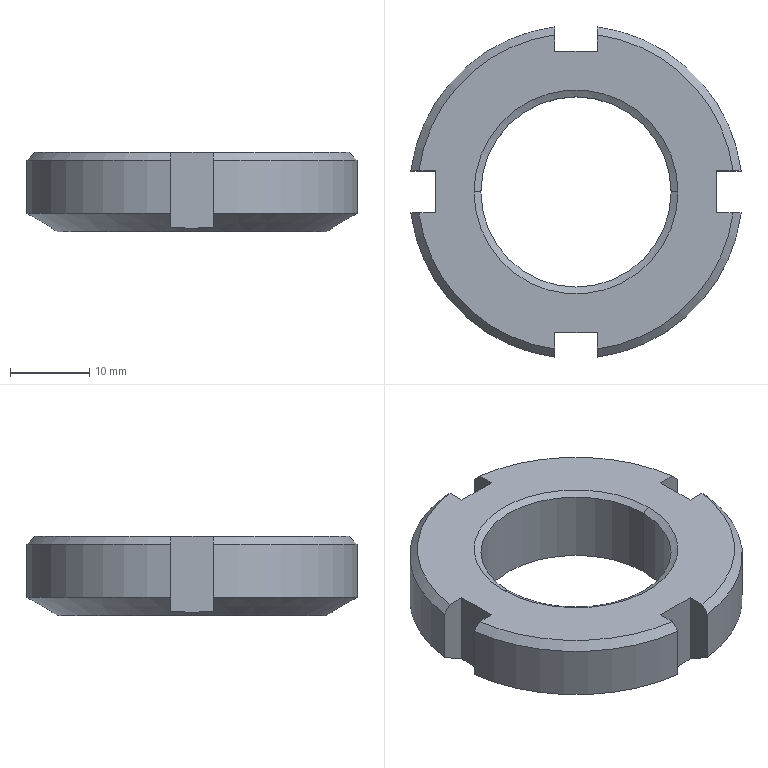Part | SolidWorks | features Chamfer 3, CirPattern 1, Cut 1, Extrusion 1 | 1 solid | 30 faces | box 41.664 x 41.664 x 10 mm | volume 8085 mm3 | plane 14 | cone 10 | cylinder 6 | commonest cylinder face diameters 42 x4 24 x2
STEP:
#1=CARTESIAN_POINT('',(-12.,0.,9.5));
#2=VERTEX_POINT('',#1);
#3=CARTESIAN_POINT('',(12.,0.,9.5));
#4=VERTEX_POINT('',#3);
#5=CARTESIAN_POINT('',(0.,0.,9.5));
#6=DIRECTION('',(0.,0.,1.));
#7=DIRECTION('',(1.,0.,0.));
#8=AXIS2_PLACEMENT_3D('',#5,#6,#7);
#9=CIRCLE('',#8,12.);
#10=EDGE_CURVE('',#2,#4,#9,.T.);
#11=ORIENTED_EDGE('',*,*,#10,.F.);
#12=CARTESIAN_POINT('',(-12.866,0.,10.));
#13=VERTEX_POINT('',#12);
#14=CARTESIAN_POINT('',(-12.,0.,9.5));
#15=DIRECTION('',(-0.866,0.,0.5));
#16=VECTOR('',#15,1000.);
#17=LINE('',#14,#16);
#18=EDGE_CURVE('',#2,#13,#17,.T.);
#19=ORIENTED_EDGE('',*,*,#18,.T.);
#20=CARTESIAN_POINT('',(12.866,0.,10.));
#21=VERTEX_POINT('',#20);
#22=CARTESIAN_POINT('',(0.,0.,10.));
#23=DIRECTION('',(0.,0.,-1.));
#24=DIRECTION('',(1.,0.,0.));
#25=AXIS2_PLACEMENT_3D('',#22,#23,#24);
#26=CIRCLE('',#25,12.866);
#27=EDGE_CURVE('',#21,#13,#26,.T.);
#28=ORIENTED_EDGE('',*,*,#27,.F.);
#29=CARTESIAN_POINT('',(12.,0.,9.5));
#30=DIRECTION('',(0.866,0.,0.5));
#31=VECTOR('',#30,1000.);
#32=LINE('',#29,#31);
#33=EDGE_CURVE('',#4,#21,#32,.T.);
#34=ORIENTED_EDGE('',*,*,#33,.F.);
#35=EDGE_LOOP('',(#11,#19,#28,#34));
#36=FACE_OUTER_BOUND('',#35,.T.);
#37=CARTESIAN_POINT('',(0.,0.,9.5));
#38=DIRECTION('',(0.,0.,1.));
#39=DIRECTION('',(1.,0.,0.));
#40=AXIS2_PLACEMENT_3D('',#37,#38,#39);
#41=CONICAL_SURFACE('',#40,12.,1.047);
#42=ADVANCED_FACE('',(#36),#41,.F.);
#43=CARTESIAN_POINT('',(12.,0.,0.5));
#44=VERTEX_POINT('',#43);
#45=CARTESIAN_POINT('',(-12.,0.,0.5));
#46=VERTEX_POINT('',#45);
#47=CARTESIAN_POINT('',(0.,0.,0.5));
#48=DIRECTION('',(0.,0.,-1.));
#49=DIRECTION('',(1.,0.,0.));
#50=AXIS2_PLACEMENT_3D('',#47,#48,#49);
#51=CIRCLE('',#50,12.);
#52=EDGE_CURVE('',#44,#46,#51,.T.);
#53=ORIENTED_EDGE('',*,*,#52,.F.);
#54=CARTESIAN_POINT('',(12.866,0.,0.));
#55=VERTEX_POINT('',#54);
#56=CARTESIAN_POINT('',(12.866,0.,0.));
#57=DIRECTION('',(0.866,0.,-0.5));
#58=VECTOR('',#57,1000.);
#59=LINE('',#56,#58);
#60=EDGE_CURVE('',#44,#55,#59,.T.);
#61=ORIENTED_EDGE('',*,*,#60,.T.);
#62=CARTESIAN_POINT('',(-12.866,0.,0.));
#63=VERTEX_POINT('',#62);
#64=CARTESIAN_POINT('',(0.,0.,0.));
#65=DIRECTION('',(0.,0.,1.));
#66=DIRECTION('',(1.,0.,0.));
#67=AXIS2_PLACEMENT_3D('',#64,#65,#66);
#68=CIRCLE('',#67,12.866);
#69=EDGE_CURVE('',#63,#55,#68,.T.);
#70=ORIENTED_EDGE('',*,*,#69,.F.);
#71=CARTESIAN_POINT('',(-12.866,0.,0.));
#72=DIRECTION('',(-0.866,0.,-0.5));
#73=VECTOR('',#72,1000.);
#74=LINE('',#71,#73);
#75=EDGE_CURVE('',#46,#63,#74,.T.);
#76=ORIENTED_EDGE('',*,*,#75,.F.);
#77=EDGE_LOOP('',(#53,#61,#70,#76));
#78=FACE_OUTER_BOUND('',#77,.T.);
#79=CARTESIAN_POINT('',(0.,0.,0.));
#80=DIRECTION('',(0.,0.,-1.));
#81=DIRECTION('',(-1.,0.,0.));
#82=AXIS2_PLACEMENT_3D('',#79,#80,#81);
#83=CONICAL_SURFACE('',#82,12.866,1.047);
#84=ADVANCED_FACE('',(#78),#83,.F.);
#85=CARTESIAN_POINT('',(-17.,0.,0.));
#86=VERTEX_POINT('',#85);
#87=CARTESIAN_POINT('',(17.,0.,0.));
#88=VERTEX_POINT('',#87);
#89=CARTESIAN_POINT('',(0.,0.,0.));
#90=DIRECTION('',(0.,0.,-1.));
#91=DIRECTION('',(1.,0.,0.));
#92=AXIS2_PLACEMENT_3D('',#89,#90,#91);
#93=CIRCLE('',#92,17.);
#94=EDGE_CURVE('',#86,#88,#93,.T.);
#95=ORIENTED_EDGE('',*,*,#94,.F.);
#96=CARTESIAN_POINT('',(-17.732,0.,0.4227));
#97=VERTEX_POINT('',#96);
#98=CARTESIAN_POINT('',(-21.,0.,2.309));
#99=DIRECTION('',(-0.866,0.,0.5));
#100=VECTOR('',#99,1000.);
#101=LINE('',#98,#100);
#102=EDGE_CURVE('',#86,#97,#101,.T.);
#103=ORIENTED_EDGE('',*,*,#102,.T.);
#104=CARTESIAN_POINT('',(-17.732,2.65,0.5364));
#105=VERTEX_POINT('',#104);
#106=CARTESIAN_POINT('',(-17.732,2.65,0.5364));
#107=CARTESIAN_POINT('',(-17.732,1.77,0.4613));
#108=CARTESIAN_POINT('',(-17.732,0.8867,0.4227));
#109=CARTESIAN_POINT('',(-17.732,0.,0.4227));
#110=B_SPLINE_CURVE_WITH_KNOTS('',3,(#106,#107,#108,#109),.UNSPECIFIED.,.F.,.F.,(4,4),(0.005044,0.007694),.UNSPECIFIED.);
#111=EDGE_CURVE('',#105,#97,#110,.T.);
#112=ORIENTED_EDGE('',*,*,#111,.F.);
#113=CARTESIAN_POINT('',(-20.832,2.65,2.309));
#114=VERTEX_POINT('',#113);
#115=CARTESIAN_POINT('',(-20.832,2.65,2.309));
#116=CARTESIAN_POINT('',(-19.799,2.65,1.718));
#117=CARTESIAN_POINT('',(-18.766,2.65,1.127));
#118=CARTESIAN_POINT('',(-17.732,2.65,0.5364));
#119=B_SPLINE_CURVE_WITH_KNOTS('',3,(#115,#116,#117,#118),.UNSPECIFIED.,.F.,.F.,(4,4),(0.00673,0.0103),.UNSPECIFIED.);
#120=EDGE_CURVE('',#114,#105,#119,.T.);
#121=ORIENTED_EDGE('',*,*,#120,.F.);
#122=CARTESIAN_POINT('',(-2.65,20.832,2.309));
#123=VERTEX_POINT('',#122);
#124=CARTESIAN_POINT('',(0.,0.,2.309));
#125=DIRECTION('',(0.,0.,1.));
#126=DIRECTION('',(1.,0.,0.));
#127=AXIS2_PLACEMENT_3D('',#124,#125,#126);
#128=CIRCLE('',#127,21.);
#129=EDGE_CURVE('',#123,#114,#128,.T.);
#130=ORIENTED_EDGE('',*,*,#129,.F.);
#131=CARTESIAN_POINT('',(-2.65,17.732,0.5364));
#132=VERTEX_POINT('',#131);
#133=CARTESIAN_POINT('',(-2.65,17.732,0.5364));
#134=CARTESIAN_POINT('',(-2.65,18.766,1.127));
#135=CARTESIAN_POINT('',(-2.65,19.799,1.718));
#136=CARTESIAN_POINT('',(-2.65,20.832,2.309));
#137=B_SPLINE_CURVE_WITH_KNOTS('',3,(#133,#134,#135,#136),.UNSPECIFIED.,.F.,.F.,(4,4),(0.006997,0.01057),.UNSPECIFIED.);
#138=EDGE_CURVE('',#132,#123,#137,.T.);
#139=ORIENTED_EDGE('',*,*,#138,.F.);
#140=CARTESIAN_POINT('',(2.65,17.732,0.5364));
#141=VERTEX_POINT('',#140);
#142=CARTESIAN_POINT('',(2.65,17.732,0.5364));
#143=CARTESIAN_POINT('',(1.773,17.732,0.4615));
#144=CARTESIAN_POINT('',(0.8926,17.732,0.423));
#145=CARTESIAN_POINT('',(-0.4329,17.732,0.4226));
#146=CARTESIAN_POINT('',(-0.8756,17.732,0.432));
#147=CARTESIAN_POINT('',(-1.763,17.732,0.47));
#148=CARTESIAN_POINT('',(-2.208,17.732,0.4986));
#149=CARTESIAN_POINT('',(-2.65,17.732,0.5364));
#150=B_SPLINE_CURVE_WITH_KNOTS('',3,(#142,#143,#144,#145,#146,#147,#148,#149),.UNSPECIFIED.,.F.,.F.,(4,2,2,4),(0.005044,0.007685,0.009006,0.01033),.UNSPECIFIED.);
#151=EDGE_CURVE('',#141,#132,#150,.T.);
#152=ORIENTED_EDGE('',*,*,#151,.F.);
#153=CARTESIAN_POINT('',(2.65,20.832,2.309));
#154=VERTEX_POINT('',#153);
#155=CARTESIAN_POINT('',(2.65,20.832,2.309));
#156=CARTESIAN_POINT('',(2.65,19.799,1.718));
#157=CARTESIAN_POINT('',(2.65,18.766,1.127));
#158=CARTESIAN_POINT('',(2.65,17.732,0.5364));
#159=B_SPLINE_CURVE_WITH_KNOTS('',3,(#155,#156,#157,#158),.UNSPECIFIED.,.F.,.F.,(4,4),(0.004139,0.00771),.UNSPECIFIED.);
#160=EDGE_CURVE('',#154,#141,#159,.T.);
#161=ORIENTED_EDGE('',*,*,#160,.F.);
#162=CARTESIAN_POINT('',(20.832,2.65,2.309));
#163=VERTEX_POINT('',#162);
#164=CARTESIAN_POINT('',(0.,0.,2.309));
#165=DIRECTION('',(0.,0.,1.));
#166=DIRECTION('',(1.,0.,0.));
#167=AXIS2_PLACEMENT_3D('',#164,#165,#166);
#168=CIRCLE('',#167,21.);
#169=EDGE_CURVE('',#163,#154,#168,.T.);
#170=ORIENTED_EDGE('',*,*,#169,.F.);
#171=CARTESIAN_POINT('',(17.732,2.65,0.5364));
#172=VERTEX_POINT('',#171);
#173=CARTESIAN_POINT('',(17.732,2.65,0.5364));
#174=CARTESIAN_POINT('',(18.766,2.65,1.127));
#175=CARTESIAN_POINT('',(19.799,2.65,1.718));
#176=CARTESIAN_POINT('',(20.832,2.65,2.309));
#177=B_SPLINE_CURVE_WITH_KNOTS('',3,(#173,#174,#175,#176),.UNSPECIFIED.,.F.,.F.,(4,4),(0.006997,0.01057),.UNSPECIFIED.);
#178=EDGE_CURVE('',#172,#163,#177,.T.);
#179=ORIENTED_EDGE('',*,*,#178,.F.);
#180=CARTESIAN_POINT('',(17.732,0.,0.4227));
#181=VERTEX_POINT('',#180);
#182=CARTESIAN_POINT('',(17.732,0.,0.4227));
#183=CARTESIAN_POINT('',(17.732,0.8867,0.4227));
#184=CARTESIAN_POINT('',(17.732,1.77,0.4613));
#185=CARTESIAN_POINT('',(17.732,2.65,0.5364));
#186=B_SPLINE_CURVE_WITH_KNOTS('',3,(#182,#183,#184,#185),.UNSPECIFIED.,.F.,.F.,(4,4),(0.01369,0.01634),.UNSPECIFIED.);
#187=EDGE_CURVE('',#181,#172,#186,.T.);
#188=ORIENTED_EDGE('',*,*,#187,.F.);
#189=CARTESIAN_POINT('',(21.,0.,2.309));
#190=DIRECTION('',(0.866,0.,0.5));
#191=VECTOR('',#190,1000.);
#192=LINE('',#189,#191);
#193=EDGE_CURVE('',#88,#181,#192,.T.);
#194=ORIENTED_EDGE('',*,*,#193,.F.);
#195=EDGE_LOOP('',(#95,#103,#112,#121,#130,#139,#152,#161,#170,#179,#188,#194));
#196=FACE_OUTER_BOUND('',#195,.T.);
#197=CARTESIAN_POINT('',(0.,0.,2.309));
#198=DIRECTION('',(0.,0.,1.));
#199=DIRECTION('',(1.,0.,0.));
#200=AXIS2_PLACEMENT_3D('',#197,#198,#199);
#201=CONICAL_SURFACE('',#200,21.,1.047);
#202=ADVANCED_FACE('',(#196),#201,.T.);
#203=ORIENTED_EDGE('',*,*,#10,.T.);
#204=CARTESIAN_POINT('',(12.,0.,10.));
#205=DIRECTION('',(0.,0.,-1.));
#206=VECTOR('',#205,1000.);
#207=LINE('',#204,#206);
#208=EDGE_CURVE('',#4,#44,#207,.T.);
#209=ORIENTED_EDGE('',*,*,#208,.T.);
#210=ORIENTED_EDGE('',*,*,#52,.T.);
#211=CARTESIAN_POINT('',(-12.,0.,10.));
#212=DIRECTION('',(0.,0.,-1.));
#213=VECTOR('',#212,1000.);
#214=LINE('',#211,#213);
#215=EDGE_CURVE('',#2,#46,#214,.T.);
#216=ORIENTED_EDGE('',*,*,#215,.F.);
#217=EDGE_LOOP('',(#203,#209,#210,#216));
#218=FACE_OUTER_BOUND('',#217,.T.);
#219=CARTESIAN_POINT('',(0.,0.,10.));
#220=DIRECTION('',(0.,0.,-1.));
#221=DIRECTION('',(-1.,0.,0.));
#222=AXIS2_PLACEMENT_3D('',#219,#220,#221);
#223=CYLINDRICAL_SURFACE('',#222,12.);
#224=ADVANCED_FACE('',(#218),#223,.F.);
#225=CARTESIAN_POINT('',(2.65,20.832,9.));
#226=VERTEX_POINT('',#225);
#227=CARTESIAN_POINT('',(20.832,2.65,9.));
#228=VERTEX_POINT('',#227);
#229=CARTESIAN_POINT('',(0.,0.,9.));
#230=DIRECTION('',(0.,0.,-1.));
#231=DIRECTION('',(1.,0.,0.));
#232=AXIS2_PLACEMENT_3D('',#229,#230,#231);
#233=CIRCLE('',#232,21.);
#234=EDGE_CURVE('',#226,#228,#233,.T.);
#235=ORIENTED_EDGE('',*,*,#234,.T.);
#236=CARTESIAN_POINT('',(20.832,2.65,0.));
#237=DIRECTION('',(0.,0.,1.));
#238=VECTOR('',#237,1000.);
#239=LINE('',#236,#238);
#240=EDGE_CURVE('',#163,#228,#239,.T.);
#241=ORIENTED_EDGE('',*,*,#240,.F.);
#242=ORIENTED_EDGE('',*,*,#169,.T.);
#243=CARTESIAN_POINT('',(2.65,20.832,0.));
#244=DIRECTION('',(0.,0.,1.));
#245=VECTOR('',#244,1000.);
#246=LINE('',#243,#245);
#247=EDGE_CURVE('',#154,#226,#246,.T.);
#248=ORIENTED_EDGE('',*,*,#247,.T.);
#249=EDGE_LOOP('',(#235,#241,#242,#248));
#250=FACE_OUTER_BOUND('',#249,.T.);
#251=CARTESIAN_POINT('',(0.,0.,10.));
#252=DIRECTION('',(0.,0.,-1.));
#253=DIRECTION('',(-1.,0.,0.));
#254=AXIS2_PLACEMENT_3D('',#251,#252,#253);
#255=CYLINDRICAL_SURFACE('',#254,21.);
#256=ADVANCED_FACE('',(#250),#255,.T.);
#257=CARTESIAN_POINT('',(19.824,2.65,10.));
#258=VERTEX_POINT('',#257);
#259=CARTESIAN_POINT('',(20.832,2.65,9.));
#260=CARTESIAN_POINT('',(20.496,2.65,9.333));
#261=CARTESIAN_POINT('',(20.16,2.65,9.667));
#262=CARTESIAN_POINT('',(19.824,2.65,10.));
#263=B_SPLINE_CURVE_WITH_KNOTS('',3,(#259,#260,#261,#262),.UNSPECIFIED.,.F.,.F.,(4,4),(0.005158,0.006578),.UNSPECIFIED.);
#264=EDGE_CURVE('',#228,#258,#263,.T.);
#265=ORIENTED_EDGE('',*,*,#264,.F.);
#266=ORIENTED_EDGE('',*,*,#234,.F.);
#267=CARTESIAN_POINT('',(2.65,19.824,10.));
#268=VERTEX_POINT('',#267);
#269=CARTESIAN_POINT('',(2.65,19.824,10.));
#270=CARTESIAN_POINT('',(2.65,20.16,9.667));
#271=CARTESIAN_POINT('',(2.65,20.496,9.333));
#272=CARTESIAN_POINT('',(2.65,20.832,9.));
#273=B_SPLINE_CURVE_WITH_KNOTS('',3,(#269,#270,#271,#272),.UNSPECIFIED.,.F.,.F.,(4,4),(0.006093,0.007513),.UNSPECIFIED.);
#274=EDGE_CURVE('',#268,#226,#273,.T.);
#275=ORIENTED_EDGE('',*,*,#274,.F.);
#276=CARTESIAN_POINT('',(0.,0.,10.));
#277=DIRECTION('',(0.,0.,1.));
#278=DIRECTION('',(1.,0.,0.));
#279=AXIS2_PLACEMENT_3D('',#276,#277,#278);
#280=CIRCLE('',#279,20.);
#281=EDGE_CURVE('',#258,#268,#280,.T.);
#282=ORIENTED_EDGE('',*,*,#281,.F.);
#283=EDGE_LOOP('',(#265,#266,#275,#282));
#284=FACE_OUTER_BOUND('',#283,.T.);
#285=CARTESIAN_POINT('',(0.,0.,10.));
#286=DIRECTION('',(0.,0.,-1.));
#287=DIRECTION('',(-1.,0.,0.));
#288=AXIS2_PLACEMENT_3D('',#285,#286,#287);
#289=CONICAL_SURFACE('',#288,20.,0.7854);
#290=ADVANCED_FACE('',(#284),#289,.T.);
#291=CARTESIAN_POINT('',(-20.832,2.65,9.));
#292=VERTEX_POINT('',#291);
#293=CARTESIAN_POINT('',(-2.65,20.832,9.));
#294=VERTEX_POINT('',#293);
#295=CARTESIAN_POINT('',(0.,0.,9.));
#296=DIRECTION('',(0.,0.,-1.));
#297=DIRECTION('',(1.,0.,0.));
#298=AXIS2_PLACEMENT_3D('',#295,#296,#297);
#299=CIRCLE('',#298,21.);
#300=EDGE_CURVE('',#292,#294,#299,.T.);
#301=ORIENTED_EDGE('',*,*,#300,.T.);
#302=CARTESIAN_POINT('',(-2.65,20.832,0.));
#303=DIRECTION('',(0.,0.,1.));
#304=VECTOR('',#303,1000.);
#305=LINE('',#302,#304);
#306=EDGE_CURVE('',#123,#294,#305,.T.);
#307=ORIENTED_EDGE('',*,*,#306,.F.);
#308=ORIENTED_EDGE('',*,*,#129,.T.);
#309=CARTESIAN_POINT('',(-20.832,2.65,0.));
#310=DIRECTION('',(0.,0.,1.));
#311=VECTOR('',#310,1000.);
#312=LINE('',#309,#311);
#313=EDGE_CURVE('',#114,#292,#312,.T.);
#314=ORIENTED_EDGE('',*,*,#313,.T.);
#315=EDGE_LOOP('',(#301,#307,#308,#314));
#316=FACE_OUTER_BOUND('',#315,.T.);
#317=CARTESIAN_POINT('',(0.,0.,10.));
#318=DIRECTION('',(0.,0.,-1.));
#319=DIRECTION('',(-1.,0.,0.));
#320=AXIS2_PLACEMENT_3D('',#317,#318,#319);
#321=CYLINDRICAL_SURFACE('',#320,21.);
#322=ADVANCED_FACE('',(#316),#321,.T.);
#323=CARTESIAN_POINT('',(-2.65,19.824,10.));
#324=VERTEX_POINT('',#323);
#325=CARTESIAN_POINT('',(-2.65,20.832,9.));
#326=CARTESIAN_POINT('',(-2.65,20.496,9.333));
#327=CARTESIAN_POINT('',(-2.65,20.16,9.667));
#328=CARTESIAN_POINT('',(-2.65,19.824,10.));
#329=B_SPLINE_CURVE_WITH_KNOTS('',3,(#325,#326,#327,#328),.UNSPECIFIED.,.F.,.F.,(4,4),(0.005158,0.006578),.UNSPECIFIED.);
#330=EDGE_CURVE('',#294,#324,#329,.T.);
#331=ORIENTED_EDGE('',*,*,#330,.F.);
#332=ORIENTED_EDGE('',*,*,#300,.F.);
#333=CARTESIAN_POINT('',(-19.824,2.65,10.));
#334=VERTEX_POINT('',#333);
#335=CARTESIAN_POINT('',(-19.824,2.65,10.));
#336=CARTESIAN_POINT('',(-20.011,2.65,9.814));
#337=CARTESIAN_POINT('',(-20.199,2.65,9.628));
#338=CARTESIAN_POINT('',(-20.387,2.65,9.442));
#339=CARTESIAN_POINT('',(-20.535,2.65,9.294));
#340=CARTESIAN_POINT('',(-20.684,2.65,9.147));
#341=CARTESIAN_POINT('',(-20.832,2.65,9.));
#342=B_SPLINE_CURVE_WITH_KNOTS('',3,(#335,#336,#337,#338,#339,#340,#341),.UNSPECIFIED.,.F.,.F.,(4,3,4),(0.005542,0.006335,0.006963),.UNSPECIFIED.);
#343=EDGE_CURVE('',#334,#292,#342,.T.);
#344=ORIENTED_EDGE('',*,*,#343,.F.);
#345=CARTESIAN_POINT('',(0.,0.,10.));
#346=DIRECTION('',(0.,0.,1.));
#347=DIRECTION('',(1.,0.,0.));
#348=AXIS2_PLACEMENT_3D('',#345,#346,#347);
#349=CIRCLE('',#348,20.);
#350=EDGE_CURVE('',#324,#334,#349,.T.);
#351=ORIENTED_EDGE('',*,*,#350,.F.);
#352=EDGE_LOOP('',(#331,#332,#344,#351));
#353=FACE_OUTER_BOUND('',#352,.T.);
#354=CARTESIAN_POINT('',(0.,0.,10.));
#355=DIRECTION('',(0.,0.,-1.));
#356=DIRECTION('',(-1.,0.,0.));
#357=AXIS2_PLACEMENT_3D('',#354,#355,#356);
#358=CONICAL_SURFACE('',#357,20.,0.7854);
#359=ADVANCED_FACE('',(#353),#358,.T.);
#360=CARTESIAN_POINT('',(-2.65,-20.832,9.));
#361=VERTEX_POINT('',#360);
#362=CARTESIAN_POINT('',(-20.832,-2.65,9.));
#363=VERTEX_POINT('',#362);
#364=CARTESIAN_POINT('',(0.,0.,9.));
#365=DIRECTION('',(0.,0.,-1.));
#366=DIRECTION('',(1.,0.,0.));
#367=AXIS2_PLACEMENT_3D('',#364,#365,#366);
#368=CIRCLE('',#367,21.);
#369=EDGE_CURVE('',#361,#363,#368,.T.);
#370=ORIENTED_EDGE('',*,*,#369,.T.);
#371=CARTESIAN_POINT('',(-20.832,-2.65,2.309));
#372=VERTEX_POINT('',#371);
#373=CARTESIAN_POINT('',(-20.832,-2.65,0.));
#374=DIRECTION('',(0.,0.,1.));
#375=VECTOR('',#374,1000.);
#376=LINE('',#373,#375);
#377=EDGE_CURVE('',#372,#363,#376,.T.);
#378=ORIENTED_EDGE('',*,*,#377,.F.);
#379=CARTESIAN_POINT('',(-2.65,-20.832,2.309));
#380=VERTEX_POINT('',#379);
#381=CARTESIAN_POINT('',(0.,0.,2.309));
#382=DIRECTION('',(0.,0.,1.));
#383=DIRECTION('',(1.,0.,0.));
#384=AXIS2_PLACEMENT_3D('',#381,#382,#383);
#385=CIRCLE('',#384,21.);
#386=EDGE_CURVE('',#372,#380,#385,.T.);
#387=ORIENTED_EDGE('',*,*,#386,.T.);
#388=CARTESIAN_POINT('',(-2.65,-20.832,0.));
#389=DIRECTION('',(0.,0.,1.));
#390=VECTOR('',#389,1000.);
#391=LINE('',#388,#390);
#392=EDGE_CURVE('',#380,#361,#391,.T.);
#393=ORIENTED_EDGE('',*,*,#392,.T.);
#394=EDGE_LOOP('',(#370,#378,#387,#393));
#395=FACE_OUTER_BOUND('',#394,.T.);
#396=CARTESIAN_POINT('',(0.,0.,10.));
#397=DIRECTION('',(0.,0.,-1.));
#398=DIRECTION('',(-1.,0.,0.));
#399=AXIS2_PLACEMENT_3D('',#396,#397,#398);
#400=CYLINDRICAL_SURFACE('',#399,21.);
#401=ADVANCED_FACE('',(#395),#400,.T.);
#402=CARTESIAN_POINT('',(-19.824,-2.65,10.));
#403=VERTEX_POINT('',#402);
#404=CARTESIAN_POINT('',(-20.832,-2.65,9.));
#405=CARTESIAN_POINT('',(-20.684,-2.65,9.147));
#406=CARTESIAN_POINT('',(-20.535,-2.65,9.294));
#407=CARTESIAN_POINT('',(-20.387,-2.65,9.442));
#408=CARTESIAN_POINT('',(-20.199,-2.65,9.628));
#409=CARTESIAN_POINT('',(-20.011,-2.65,9.814));
#410=CARTESIAN_POINT('',(-19.824,-2.65,10.));
#411=B_SPLINE_CURVE_WITH_KNOTS('',3,(#404,#405,#406,#407,#408,#409,#410),.UNSPECIFIED.,.F.,.F.,(4,3,4),(0.005708,0.006335,0.007128),.UNSPECIFIED.);
#412=EDGE_CURVE('',#363,#403,#411,.T.);
#413=ORIENTED_EDGE('',*,*,#412,.F.);
#414=ORIENTED_EDGE('',*,*,#369,.F.);
#415=CARTESIAN_POINT('',(-2.65,-19.824,10.));
#416=VERTEX_POINT('',#415);
#417=CARTESIAN_POINT('',(-2.65,-19.824,10.));
#418=CARTESIAN_POINT('',(-2.65,-20.011,9.814));
#419=CARTESIAN_POINT('',(-2.65,-20.199,9.628));
#420=CARTESIAN_POINT('',(-2.65,-20.387,9.442));
#421=CARTESIAN_POINT('',(-2.65,-20.535,9.294));
#422=CARTESIAN_POINT('',(-2.65,-20.684,9.147));
#423=CARTESIAN_POINT('',(-2.65,-20.832,9.));
#424=B_SPLINE_CURVE_WITH_KNOTS('',3,(#417,#418,#419,#420,#421,#422,#423),.UNSPECIFIED.,.F.,.F.,(4,3,4),(0.005542,0.006335,0.006963),.UNSPECIFIED.);
#425=EDGE_CURVE('',#416,#361,#424,.T.);
#426=ORIENTED_EDGE('',*,*,#425,.F.);
#427=CARTESIAN_POINT('',(0.,0.,10.));
#428=DIRECTION('',(0.,0.,1.));
#429=DIRECTION('',(1.,0.,0.));
#430=AXIS2_PLACEMENT_3D('',#427,#428,#429);
#431=CIRCLE('',#430,20.);
#432=EDGE_CURVE('',#403,#416,#431,.T.);
#433=ORIENTED_EDGE('',*,*,#432,.F.);
#434=EDGE_LOOP('',(#413,#414,#426,#433));
#435=FACE_OUTER_BOUND('',#434,.T.);
#436=CARTESIAN_POINT('',(0.,0.,10.));
#437=DIRECTION('',(0.,0.,-1.));
#438=DIRECTION('',(-1.,0.,0.));
#439=AXIS2_PLACEMENT_3D('',#436,#437,#438);
#440=CONICAL_SURFACE('',#439,20.,0.7854);
#441=ADVANCED_FACE('',(#435),#440,.T.);
#442=ORIENTED_EDGE('',*,*,#27,.T.);
#443=CARTESIAN_POINT('',(0.,0.,10.));
#444=DIRECTION('',(0.,0.,-1.));
#445=DIRECTION('',(1.,0.,0.));
#446=AXIS2_PLACEMENT_3D('',#443,#444,#445);
#447=CIRCLE('',#446,12.866);
#448=EDGE_CURVE('',#13,#21,#447,.T.);
#449=ORIENTED_EDGE('',*,*,#448,.T.);
#450=EDGE_LOOP('',(#442,#449));
#451=FACE_BOUND('',#450,.T.);
#452=CARTESIAN_POINT('',(17.732,2.65,10.));
#453=VERTEX_POINT('',#452);
#454=CARTESIAN_POINT('',(17.732,2.65,10.));
#455=DIRECTION('',(-1.,0.,0.));
#456=VECTOR('',#455,1000.);
#457=LINE('',#454,#456);
#458=EDGE_CURVE('',#258,#453,#457,.T.);
#459=ORIENTED_EDGE('',*,*,#458,.F.);
#460=ORIENTED_EDGE('',*,*,#281,.T.);
#461=CARTESIAN_POINT('',(2.65,17.732,10.));
#462=VERTEX_POINT('',#461);
#463=CARTESIAN_POINT('',(2.65,17.732,10.));
#464=DIRECTION('',(0.,1.,0.));
#465=VECTOR('',#464,1000.);
#466=LINE('',#463,#465);
#467=EDGE_CURVE('',#462,#268,#466,.T.);
#468=ORIENTED_EDGE('',*,*,#467,.F.);
#469=CARTESIAN_POINT('',(-2.65,17.732,10.));
#470=VERTEX_POINT('',#469);
#471=CARTESIAN_POINT('',(2.65,17.732,10.));
#472=DIRECTION('',(1.,0.,0.));
#473=VECTOR('',#472,1000.);
#474=LINE('',#471,#473);
#475=EDGE_CURVE('',#470,#462,#474,.T.);
#476=ORIENTED_EDGE('',*,*,#475,.F.);
#477=CARTESIAN_POINT('',(-2.65,17.732,10.));
#478=DIRECTION('',(0.,-1.,0.));
#479=VECTOR('',#478,1000.);
#480=LINE('',#477,#479);
#481=EDGE_CURVE('',#324,#470,#480,.T.);
#482=ORIENTED_EDGE('',*,*,#481,.F.);
#483=ORIENTED_EDGE('',*,*,#350,.T.);
#484=CARTESIAN_POINT('',(-17.732,2.65,10.));
#485=VERTEX_POINT('',#484);
#486=CARTESIAN_POINT('',(-17.732,2.65,10.));
#487=DIRECTION('',(-1.,0.,0.));
#488=VECTOR('',#487,1000.);
#489=LINE('',#486,#488);
#490=EDGE_CURVE('',#485,#334,#489,.T.);
#491=ORIENTED_EDGE('',*,*,#490,.F.);
#492=CARTESIAN_POINT('',(-17.732,-2.65,10.));
#493=VERTEX_POINT('',#492);
#494=CARTESIAN_POINT('',(-17.732,2.65,10.));
#495=DIRECTION('',(0.,1.,0.));
#496=VECTOR('',#495,1000.);
#497=LINE('',#494,#496);
#498=EDGE_CURVE('',#493,#485,#497,.T.);
#499=ORIENTED_EDGE('',*,*,#498,.F.);
#500=CARTESIAN_POINT('',(-17.732,-2.65,10.));
#501=DIRECTION('',(1.,0.,0.));
#502=VECTOR('',#501,1000.);
#503=LINE('',#500,#502);
#504=EDGE_CURVE('',#403,#493,#503,.T.);
#505=ORIENTED_EDGE('',*,*,#504,.F.);
#506=ORIENTED_EDGE('',*,*,#432,.T.);
#507=CARTESIAN_POINT('',(-2.65,-17.732,10.));
#508=VERTEX_POINT('',#507);
#509=CARTESIAN_POINT('',(-2.65,-17.732,10.));
#510=DIRECTION('',(0.,-1.,0.));
#511=VECTOR('',#510,1000.);
#512=LINE('',#509,#511);
#513=EDGE_CURVE('',#508,#416,#512,.T.);
#514=ORIENTED_EDGE('',*,*,#513,.F.);
#515=CARTESIAN_POINT('',(2.65,-17.732,10.));
#516=VERTEX_POINT('',#515);
#517=CARTESIAN_POINT('',(-2.65,-17.732,10.));
#518=DIRECTION('',(-1.,0.,0.));
#519=VECTOR('',#518,1000.);
#520=LINE('',#517,#519);
#521=EDGE_CURVE('',#516,#508,#520,.T.);
#522=ORIENTED_EDGE('',*,*,#521,.F.);
#523=CARTESIAN_POINT('',(2.65,-19.824,10.));
#524=VERTEX_POINT('',#523);
#525=CARTESIAN_POINT('',(2.65,-17.732,10.));
#526=DIRECTION('',(0.,1.,0.));
#527=VECTOR('',#526,1000.);
#528=LINE('',#525,#527);
#529=EDGE_CURVE('',#524,#516,#528,.T.);
#530=ORIENTED_EDGE('',*,*,#529,.F.);
#531=CARTESIAN_POINT('',(19.824,-2.65,10.));
#532=VERTEX_POINT('',#531);
#533=CARTESIAN_POINT('',(0.,0.,10.));
#534=DIRECTION('',(0.,0.,1.));
#535=DIRECTION('',(1.,0.,0.));
#536=AXIS2_PLACEMENT_3D('',#533,#534,#535);
#537=CIRCLE('',#536,20.);
#538=EDGE_CURVE('',#524,#532,#537,.T.);
#539=ORIENTED_EDGE('',*,*,#538,.T.);
#540=CARTESIAN_POINT('',(17.732,-2.65,10.));
#541=VERTEX_POINT('',#540);
#542=CARTESIAN_POINT('',(17.732,-2.65,10.));
#543=DIRECTION('',(1.,0.,0.));
#544=VECTOR('',#543,1000.);
#545=LINE('',#542,#544);
#546=EDGE_CURVE('',#541,#532,#545,.T.);
#547=ORIENTED_EDGE('',*,*,#546,.F.);
#548=CARTESIAN_POINT('',(17.732,-2.65,10.));
#549=DIRECTION('',(0.,-1.,0.));
#550=VECTOR('',#549,1000.);
#551=LINE('',#548,#550);
#552=EDGE_CURVE('',#453,#541,#551,.T.);
#553=ORIENTED_EDGE('',*,*,#552,.F.);
#554=EDGE_LOOP('',(#459,#460,#468,#476,#482,#483,#491,#499,#505,#506,#514,#522,#530,#539,#547,#553));
#555=FACE_OUTER_BOUND('',#554,.T.);
#556=CARTESIAN_POINT('',(0.,0.,10.));
#557=DIRECTION('',(0.,0.,1.));
#558=DIRECTION('',(1.,0.,0.));
#559=AXIS2_PLACEMENT_3D('',#556,#557,#558);
#560=PLANE('',#559);
#561=ADVANCED_FACE('',(#451,#555),#560,.T.);
#562=ORIENTED_EDGE('',*,*,#69,.T.);
#563=CARTESIAN_POINT('',(0.,0.,0.));
#564=DIRECTION('',(0.,0.,1.));
#565=DIRECTION('',(1.,0.,0.));
#566=AXIS2_PLACEMENT_3D('',#563,#564,#565);
#567=CIRCLE('',#566,12.866);
#568=EDGE_CURVE('',#55,#63,#567,.T.);
#569=ORIENTED_EDGE('',*,*,#568,.T.);
#570=EDGE_LOOP('',(#562,#569));
#571=FACE_BOUND('',#570,.T.);
#572=CARTESIAN_POINT('',(0.,0.,0.));
#573=DIRECTION('',(0.,0.,-1.));
#574=DIRECTION('',(1.,0.,0.));
#575=AXIS2_PLACEMENT_3D('',#572,#573,#574);
#576=CIRCLE('',#575,17.);
#577=EDGE_CURVE('',#88,#86,#576,.T.);
#578=ORIENTED_EDGE('',*,*,#577,.T.);
#579=ORIENTED_EDGE('',*,*,#94,.T.);
#580=EDGE_LOOP('',(#578,#579));
#581=FACE_OUTER_BOUND('',#580,.T.);
#582=CARTESIAN_POINT('',(0.,0.,0.));
#583=DIRECTION('',(0.,0.,1.));
#584=DIRECTION('',(1.,0.,0.));
#585=AXIS2_PLACEMENT_3D('',#582,#583,#584);
#586=PLANE('',#585);
#587=ADVANCED_FACE('',(#571,#581),#586,.F.);
#588=CARTESIAN_POINT('',(2.65,-20.832,2.309));
#589=VERTEX_POINT('',#588);
#590=CARTESIAN_POINT('',(20.832,-2.65,2.309));
#591=VERTEX_POINT('',#590);
#592=CARTESIAN_POINT('',(0.,0.,2.309));
#593=DIRECTION('',(0.,0.,1.));
#594=DIRECTION('',(1.,0.,0.));
#595=AXIS2_PLACEMENT_3D('',#592,#593,#594);
#596=CIRCLE('',#595,21.);
#597=EDGE_CURVE('',#589,#591,#596,.T.);
#598=ORIENTED_EDGE('',*,*,#597,.T.);
#599=CARTESIAN_POINT('',(20.832,-2.65,9.));
#600=VERTEX_POINT('',#599);
#601=CARTESIAN_POINT('',(20.832,-2.65,0.));
#602=DIRECTION('',(0.,0.,1.));
#603=VECTOR('',#602,1000.);
#604=LINE('',#601,#603);
#605=EDGE_CURVE('',#591,#600,#604,.T.);
#606=ORIENTED_EDGE('',*,*,#605,.T.);
#607=CARTESIAN_POINT('',(2.65,-20.832,9.));
#608=VERTEX_POINT('',#607);
#609=CARTESIAN_POINT('',(0.,0.,9.));
#610=DIRECTION('',(0.,0.,-1.));
#611=DIRECTION('',(1.,0.,0.));
#612=AXIS2_PLACEMENT_3D('',#609,#610,#611);
#613=CIRCLE('',#612,21.);
#614=EDGE_CURVE('',#600,#608,#613,.T.);
#615=ORIENTED_EDGE('',*,*,#614,.T.);
#616=CARTESIAN_POINT('',(2.65,-20.832,0.));
#617=DIRECTION('',(0.,0.,1.));
#618=VECTOR('',#617,1000.);
#619=LINE('',#616,#618);
#620=EDGE_CURVE('',#589,#608,#619,.T.);
#621=ORIENTED_EDGE('',*,*,#620,.F.);
#622=EDGE_LOOP('',(#598,#606,#615,#621));
#623=FACE_OUTER_BOUND('',#622,.T.);
#624=CARTESIAN_POINT('',(0.,0.,10.));
#625=DIRECTION('',(0.,0.,-1.));
#626=DIRECTION('',(-1.,0.,0.));
#627=AXIS2_PLACEMENT_3D('',#624,#625,#626);
#628=CYLINDRICAL_SURFACE('',#627,21.);
#629=ADVANCED_FACE('',(#623),#628,.T.);
#630=ORIENTED_EDGE('',*,*,#208,.F.);
#631=CARTESIAN_POINT('',(0.,0.,9.5));
#632=DIRECTION('',(0.,0.,1.));
#633=DIRECTION('',(1.,0.,0.));
#634=AXIS2_PLACEMENT_3D('',#631,#632,#633);
#635=CIRCLE('',#634,12.);
#636=EDGE_CURVE('',#4,#2,#635,.T.);
#637=ORIENTED_EDGE('',*,*,#636,.T.);
#638=ORIENTED_EDGE('',*,*,#215,.T.);
#639=CARTESIAN_POINT('',(0.,0.,0.5));
#640=DIRECTION('',(0.,0.,-1.));
#641=DIRECTION('',(1.,0.,0.));
#642=AXIS2_PLACEMENT_3D('',#639,#640,#641);
#643=CIRCLE('',#642,12.);
#644=EDGE_CURVE('',#46,#44,#643,.T.);
#645=ORIENTED_EDGE('',*,*,#644,.T.);
#646=EDGE_LOOP('',(#630,#637,#638,#645));
#647=FACE_OUTER_BOUND('',#646,.T.);
#648=CARTESIAN_POINT('',(0.,0.,10.));
#649=DIRECTION('',(0.,0.,-1.));
#650=DIRECTION('',(-1.,0.,0.));
#651=AXIS2_PLACEMENT_3D('',#648,#649,#650);
#652=CYLINDRICAL_SURFACE('',#651,12.);
#653=ADVANCED_FACE('',(#647),#652,.F.);
#654=CARTESIAN_POINT('',(19.824,-2.65,10.));
#655=CARTESIAN_POINT('',(20.16,-2.65,9.667));
#656=CARTESIAN_POINT('',(20.496,-2.65,9.333));
#657=CARTESIAN_POINT('',(20.832,-2.65,9.));
#658=B_SPLINE_CURVE_WITH_KNOTS('',3,(#654,#655,#656,#657),.UNSPECIFIED.,.F.,.F.,(4,4),(0.006093,0.007513),.UNSPECIFIED.);
#659=EDGE_CURVE('',#532,#600,#658,.T.);
#660=ORIENTED_EDGE('',*,*,#659,.F.);
#661=ORIENTED_EDGE('',*,*,#538,.F.);
#662=CARTESIAN_POINT('',(2.65,-20.832,9.));
#663=CARTESIAN_POINT('',(2.65,-20.684,9.147));
#664=CARTESIAN_POINT('',(2.65,-20.535,9.294));
#665=CARTESIAN_POINT('',(2.65,-20.387,9.442));
#666=CARTESIAN_POINT('',(2.65,-20.199,9.628));
#667=CARTESIAN_POINT('',(2.65,-20.011,9.814));
#668=CARTESIAN_POINT('',(2.65,-19.824,10.));
#669=B_SPLINE_CURVE_WITH_KNOTS('',3,(#662,#663,#664,#665,#666,#667,#668),.UNSPECIFIED.,.F.,.F.,(4,3,4),(0.005708,0.006335,0.007128),.UNSPECIFIED.);
#670=EDGE_CURVE('',#608,#524,#669,.T.);
#671=ORIENTED_EDGE('',*,*,#670,.F.);
#672=ORIENTED_EDGE('',*,*,#614,.F.);
#673=EDGE_LOOP('',(#660,#661,#671,#672));
#674=FACE_OUTER_BOUND('',#673,.T.);
#675=CARTESIAN_POINT('',(0.,0.,10.));
#676=DIRECTION('',(0.,0.,-1.));
#677=DIRECTION('',(-1.,0.,0.));
#678=AXIS2_PLACEMENT_3D('',#675,#676,#677);
#679=CONICAL_SURFACE('',#678,20.,0.7854);
#680=ADVANCED_FACE('',(#674),#679,.T.);
#681=ORIENTED_EDGE('',*,*,#102,.F.);
#682=ORIENTED_EDGE('',*,*,#577,.F.);
#683=ORIENTED_EDGE('',*,*,#193,.T.);
#684=CARTESIAN_POINT('',(17.732,-2.65,0.5364));
#685=VERTEX_POINT('',#684);
#686=CARTESIAN_POINT('',(17.732,-2.65,0.5364));
#687=CARTESIAN_POINT('',(17.732,-2.209,0.4988));
#688=CARTESIAN_POINT('',(17.732,-1.766,0.4702));
#689=CARTESIAN_POINT('',(17.732,-0.8815,0.4322));
#690=CARTESIAN_POINT('',(17.732,-0.4404,0.4227));
#691=CARTESIAN_POINT('',(17.732,0.,0.4227));
#692=B_SPLINE_CURVE_WITH_KNOTS('',3,(#686,#687,#688,#689,#690,#691),.UNSPECIFIED.,.F.,.F.,(4,2,4),(0.01106,0.01237,0.01369),.UNSPECIFIED.);
#693=EDGE_CURVE('',#685,#181,#692,.T.);
#694=ORIENTED_EDGE('',*,*,#693,.F.);
#695=CARTESIAN_POINT('',(20.832,-2.65,2.309));
#696=CARTESIAN_POINT('',(19.799,-2.65,1.718));
#697=CARTESIAN_POINT('',(18.766,-2.65,1.127));
#698=CARTESIAN_POINT('',(17.732,-2.65,0.5364));
#699=B_SPLINE_CURVE_WITH_KNOTS('',3,(#695,#696,#697,#698),.UNSPECIFIED.,.F.,.F.,(4,4),(0.004139,0.00771),.UNSPECIFIED.);
#700=EDGE_CURVE('',#591,#685,#699,.T.);
#701=ORIENTED_EDGE('',*,*,#700,.F.);
#702=ORIENTED_EDGE('',*,*,#597,.F.);
#703=CARTESIAN_POINT('',(2.65,-17.732,0.5364));
#704=VERTEX_POINT('',#703);
#705=CARTESIAN_POINT('',(2.65,-17.732,0.5364));
#706=CARTESIAN_POINT('',(2.65,-18.766,1.127));
#707=CARTESIAN_POINT('',(2.65,-19.799,1.718));
#708=CARTESIAN_POINT('',(2.65,-20.832,2.309));
#709=B_SPLINE_CURVE_WITH_KNOTS('',3,(#705,#706,#707,#708),.UNSPECIFIED.,.F.,.F.,(4,4),(0.004406,0.007977),.UNSPECIFIED.);
#710=EDGE_CURVE('',#704,#589,#709,.T.);
#711=ORIENTED_EDGE('',*,*,#710,.F.);
#712=CARTESIAN_POINT('',(-2.65,-17.732,0.5364));
#713=VERTEX_POINT('',#712);
#714=CARTESIAN_POINT('',(-2.65,-17.732,0.5364));
#715=CARTESIAN_POINT('',(-2.208,-17.732,0.4986));
#716=CARTESIAN_POINT('',(-1.763,-17.732,0.47));
#717=CARTESIAN_POINT('',(-0.8756,-17.732,0.432));
#718=CARTESIAN_POINT('',(-0.4329,-17.732,0.4226));
#719=CARTESIAN_POINT('',(0.8926,-17.732,0.423));
#720=CARTESIAN_POINT('',(1.773,-17.732,0.4615));
#721=CARTESIAN_POINT('',(2.65,-17.732,0.5364));
#722=B_SPLINE_CURVE_WITH_KNOTS('',3,(#714,#715,#716,#717,#718,#719,#720,#721),.UNSPECIFIED.,.F.,.F.,(4,2,2,4),(0.01106,0.01238,0.0137,0.01634),.UNSPECIFIED.);
#723=EDGE_CURVE('',#713,#704,#722,.T.);
#724=ORIENTED_EDGE('',*,*,#723,.F.);
#725=CARTESIAN_POINT('',(-2.65,-20.832,2.309));
#726=CARTESIAN_POINT('',(-2.65,-19.799,1.718));
#727=CARTESIAN_POINT('',(-2.65,-18.766,1.127));
#728=CARTESIAN_POINT('',(-2.65,-17.732,0.5364));
#729=B_SPLINE_CURVE_WITH_KNOTS('',3,(#725,#726,#727,#728),.UNSPECIFIED.,.F.,.F.,(4,4),(0.00673,0.0103),.UNSPECIFIED.);
#730=EDGE_CURVE('',#380,#713,#729,.T.);
#731=ORIENTED_EDGE('',*,*,#730,.F.);
#732=ORIENTED_EDGE('',*,*,#386,.F.);
#733=CARTESIAN_POINT('',(-17.732,-2.65,0.5364));
#734=VERTEX_POINT('',#733);
#735=CARTESIAN_POINT('',(-17.732,-2.65,0.5364));
#736=CARTESIAN_POINT('',(-18.766,-2.65,1.127));
#737=CARTESIAN_POINT('',(-19.799,-2.65,1.718));
#738=CARTESIAN_POINT('',(-20.832,-2.65,2.309));
#739=B_SPLINE_CURVE_WITH_KNOTS('',3,(#735,#736,#737,#738),.UNSPECIFIED.,.F.,.F.,(4,4),(0.004406,0.007977),.UNSPECIFIED.);
#740=EDGE_CURVE('',#734,#372,#739,.T.);
#741=ORIENTED_EDGE('',*,*,#740,.F.);
#742=CARTESIAN_POINT('',(-17.732,0.,0.4227));
#743=CARTESIAN_POINT('',(-17.732,-0.4404,0.4227));
#744=CARTESIAN_POINT('',(-17.732,-0.8815,0.4322));
#745=CARTESIAN_POINT('',(-17.732,-1.766,0.4702));
#746=CARTESIAN_POINT('',(-17.732,-2.209,0.4988));
#747=CARTESIAN_POINT('',(-17.732,-2.65,0.5364));
#748=B_SPLINE_CURVE_WITH_KNOTS('',3,(#742,#743,#744,#745,#746,#747),.UNSPECIFIED.,.F.,.F.,(4,2,4),(0.007694,0.00901,0.01033),.UNSPECIFIED.);
#749=EDGE_CURVE('',#97,#734,#748,.T.);
#750=ORIENTED_EDGE('',*,*,#749,.F.);
#751=EDGE_LOOP('',(#681,#682,#683,#694,#701,#702,#711,#724,#731,#732,#741,#750));
#752=FACE_OUTER_BOUND('',#751,.T.);
#753=CARTESIAN_POINT('',(0.,0.,2.309));
#754=DIRECTION('',(0.,0.,1.));
#755=DIRECTION('',(1.,0.,0.));
#756=AXIS2_PLACEMENT_3D('',#753,#754,#755);
#757=CONICAL_SURFACE('',#756,21.,1.047);
#758=ADVANCED_FACE('',(#752),#757,.T.);
#759=ORIENTED_EDGE('',*,*,#723,.T.);
#760=CARTESIAN_POINT('',(2.65,-17.732,0.));
#761=DIRECTION('',(0.,0.,1.));
#762=VECTOR('',#761,1000.);
#763=LINE('',#760,#762);
#764=EDGE_CURVE('',#704,#516,#763,.T.);
#765=ORIENTED_EDGE('',*,*,#764,.T.);
#766=ORIENTED_EDGE('',*,*,#521,.T.);
#767=CARTESIAN_POINT('',(-2.65,-17.732,0.));
#768=DIRECTION('',(0.,0.,1.));
#769=VECTOR('',#768,1000.);
#770=LINE('',#767,#769);
#771=EDGE_CURVE('',#713,#508,#770,.T.);
#772=ORIENTED_EDGE('',*,*,#771,.F.);
#773=EDGE_LOOP('',(#759,#765,#766,#772));
#774=FACE_OUTER_BOUND('',#773,.T.);
#775=CARTESIAN_POINT('',(-2.65,-17.732,0.));
#776=DIRECTION('',(0.,1.,0.));
#777=DIRECTION('',(0.,0.,1.));
#778=AXIS2_PLACEMENT_3D('',#775,#776,#777);
#779=PLANE('',#778);
#780=ADVANCED_FACE('',(#774),#779,.F.);
#781=ORIENTED_EDGE('',*,*,#670,.T.);
#782=ORIENTED_EDGE('',*,*,#529,.T.);
#783=ORIENTED_EDGE('',*,*,#764,.F.);
#784=ORIENTED_EDGE('',*,*,#710,.T.);
#785=ORIENTED_EDGE('',*,*,#620,.T.);
#786=EDGE_LOOP('',(#781,#782,#783,#784,#785));
#787=FACE_OUTER_BOUND('',#786,.T.);
#788=CARTESIAN_POINT('',(2.65,-17.732,0.));
#789=DIRECTION('',(1.,0.,0.));
#790=DIRECTION('',(0.,1.,0.));
#791=AXIS2_PLACEMENT_3D('',#788,#789,#790);
#792=PLANE('',#791);
#793=ADVANCED_FACE('',(#787),#792,.F.);
#794=ORIENTED_EDGE('',*,*,#425,.T.);
#795=ORIENTED_EDGE('',*,*,#392,.F.);
#796=ORIENTED_EDGE('',*,*,#730,.T.);
#797=ORIENTED_EDGE('',*,*,#771,.T.);
#798=ORIENTED_EDGE('',*,*,#513,.T.);
#799=EDGE_LOOP('',(#794,#795,#796,#797,#798));
#800=FACE_OUTER_BOUND('',#799,.T.);
#801=CARTESIAN_POINT('',(-2.65,-17.732,0.));
#802=DIRECTION('',(-1.,0.,0.));
#803=DIRECTION('',(0.,-1.,0.));
#804=AXIS2_PLACEMENT_3D('',#801,#802,#803);
#805=PLANE('',#804);
#806=ADVANCED_FACE('',(#800),#805,.F.);
#807=ORIENTED_EDGE('',*,*,#111,.T.);
#808=ORIENTED_EDGE('',*,*,#749,.T.);
#809=CARTESIAN_POINT('',(-17.732,-2.65,0.));
#810=DIRECTION('',(0.,0.,1.));
#811=VECTOR('',#810,1000.);
#812=LINE('',#809,#811);
#813=EDGE_CURVE('',#734,#493,#812,.T.);
#814=ORIENTED_EDGE('',*,*,#813,.T.);
#815=ORIENTED_EDGE('',*,*,#498,.T.);
#816=CARTESIAN_POINT('',(-17.732,2.65,0.));
#817=DIRECTION('',(0.,0.,1.));
#818=VECTOR('',#817,1000.);
#819=LINE('',#816,#818);
#820=EDGE_CURVE('',#105,#485,#819,.T.);
#821=ORIENTED_EDGE('',*,*,#820,.F.);
#822=EDGE_LOOP('',(#807,#808,#814,#815,#821));
#823=FACE_OUTER_BOUND('',#822,.T.);
#824=CARTESIAN_POINT('',(-17.732,2.65,0.));
#825=DIRECTION('',(1.,0.,0.));
#826=DIRECTION('',(0.,1.,0.));
#827=AXIS2_PLACEMENT_3D('',#824,#825,#826);
#828=PLANE('',#827);
#829=ADVANCED_FACE('',(#823),#828,.F.);
#830=ORIENTED_EDGE('',*,*,#412,.T.);
#831=ORIENTED_EDGE('',*,*,#504,.T.);
#832=ORIENTED_EDGE('',*,*,#813,.F.);
#833=ORIENTED_EDGE('',*,*,#740,.T.);
#834=ORIENTED_EDGE('',*,*,#377,.T.);
#835=EDGE_LOOP('',(#830,#831,#832,#833,#834));
#836=FACE_OUTER_BOUND('',#835,.T.);
#837=CARTESIAN_POINT('',(-17.732,-2.65,0.));
#838=DIRECTION('',(0.,-1.,0.));
#839=DIRECTION('',(1.,0.,0.));
#840=AXIS2_PLACEMENT_3D('',#837,#838,#839);
#841=PLANE('',#840);
#842=ADVANCED_FACE('',(#836),#841,.F.);
#843=ORIENTED_EDGE('',*,*,#343,.T.);
#844=ORIENTED_EDGE('',*,*,#313,.F.);
#845=ORIENTED_EDGE('',*,*,#120,.T.);
#846=ORIENTED_EDGE('',*,*,#820,.T.);
#847=ORIENTED_EDGE('',*,*,#490,.T.);
#848=EDGE_LOOP('',(#843,#844,#845,#846,#847));
#849=FACE_OUTER_BOUND('',#848,.T.);
#850=CARTESIAN_POINT('',(-17.732,2.65,0.));
#851=DIRECTION('',(0.,1.,0.));
#852=DIRECTION('',(-1.,0.,0.));
#853=AXIS2_PLACEMENT_3D('',#850,#851,#852);
#854=PLANE('',#853);
#855=ADVANCED_FACE('',(#849),#854,.F.);
#856=ORIENTED_EDGE('',*,*,#151,.T.);
#857=CARTESIAN_POINT('',(-2.65,17.732,0.));
#858=DIRECTION('',(0.,0.,1.));
#859=VECTOR('',#858,1000.);
#860=LINE('',#857,#859);
#861=EDGE_CURVE('',#132,#470,#860,.T.);
#862=ORIENTED_EDGE('',*,*,#861,.T.);
#863=ORIENTED_EDGE('',*,*,#475,.T.);
#864=CARTESIAN_POINT('',(2.65,17.732,0.));
#865=DIRECTION('',(0.,0.,1.));
#866=VECTOR('',#865,1000.);
#867=LINE('',#864,#866);
#868=EDGE_CURVE('',#141,#462,#867,.T.);
#869=ORIENTED_EDGE('',*,*,#868,.F.);
#870=EDGE_LOOP('',(#856,#862,#863,#869));
#871=FACE_OUTER_BOUND('',#870,.T.);
#872=CARTESIAN_POINT('',(2.65,17.732,0.));
#873=DIRECTION('',(0.,-1.,0.));
#874=DIRECTION('',(1.,0.,0.));
#875=AXIS2_PLACEMENT_3D('',#872,#873,#874);
#876=PLANE('',#875);
#877=ADVANCED_FACE('',(#871),#876,.F.);
#878=ORIENTED_EDGE('',*,*,#330,.T.);
#879=ORIENTED_EDGE('',*,*,#481,.T.);
#880=ORIENTED_EDGE('',*,*,#861,.F.);
#881=ORIENTED_EDGE('',*,*,#138,.T.);
#882=ORIENTED_EDGE('',*,*,#306,.T.);
#883=EDGE_LOOP('',(#878,#879,#880,#881,#882));
#884=FACE_OUTER_BOUND('',#883,.T.);
#885=CARTESIAN_POINT('',(-2.65,17.732,0.));
#886=DIRECTION('',(-1.,0.,0.));
#887=DIRECTION('',(0.,-1.,0.));
#888=AXIS2_PLACEMENT_3D('',#885,#886,#887);
#889=PLANE('',#888);
#890=ADVANCED_FACE('',(#884),#889,.F.);
#891=ORIENTED_EDGE('',*,*,#274,.T.);
#892=ORIENTED_EDGE('',*,*,#247,.F.);
#893=ORIENTED_EDGE('',*,*,#160,.T.);
#894=ORIENTED_EDGE('',*,*,#868,.T.);
#895=ORIENTED_EDGE('',*,*,#467,.T.);
#896=EDGE_LOOP('',(#891,#892,#893,#894,#895));
#897=FACE_OUTER_BOUND('',#896,.T.);
#898=CARTESIAN_POINT('',(2.65,17.732,0.));
#899=DIRECTION('',(1.,0.,0.));
#900=DIRECTION('',(0.,1.,0.));
#901=AXIS2_PLACEMENT_3D('',#898,#899,#900);
#902=PLANE('',#901);
#903=ADVANCED_FACE('',(#897),#902,.F.);
#904=ORIENTED_EDGE('',*,*,#693,.T.);
#905=ORIENTED_EDGE('',*,*,#187,.T.);
#906=CARTESIAN_POINT('',(17.732,2.65,0.));
#907=DIRECTION('',(0.,0.,1.));
#908=VECTOR('',#907,1000.);
#909=LINE('',#906,#908);
#910=EDGE_CURVE('',#172,#453,#909,.T.);
#911=ORIENTED_EDGE('',*,*,#910,.T.);
#912=ORIENTED_EDGE('',*,*,#552,.T.);
#913=CARTESIAN_POINT('',(17.732,-2.65,0.));
#914=DIRECTION('',(0.,0.,1.));
#915=VECTOR('',#914,1000.);
#916=LINE('',#913,#915);
#917=EDGE_CURVE('',#685,#541,#916,.T.);
#918=ORIENTED_EDGE('',*,*,#917,.F.);
#919=EDGE_LOOP('',(#904,#905,#911,#912,#918));
#920=FACE_OUTER_BOUND('',#919,.T.);
#921=CARTESIAN_POINT('',(17.732,-2.65,0.));
#922=DIRECTION('',(-1.,0.,0.));
#923=DIRECTION('',(0.,-1.,0.));
#924=AXIS2_PLACEMENT_3D('',#921,#922,#923);
#925=PLANE('',#924);
#926=ADVANCED_FACE('',(#920),#925,.F.);
#927=ORIENTED_EDGE('',*,*,#264,.T.);
#928=ORIENTED_EDGE('',*,*,#458,.T.);
#929=ORIENTED_EDGE('',*,*,#910,.F.);
#930=ORIENTED_EDGE('',*,*,#178,.T.);
#931=ORIENTED_EDGE('',*,*,#240,.T.);
#932=EDGE_LOOP('',(#927,#928,#929,#930,#931));
#933=FACE_OUTER_BOUND('',#932,.T.);
#934=CARTESIAN_POINT('',(17.732,2.65,0.));
#935=DIRECTION('',(0.,1.,0.));
#936=DIRECTION('',(-1.,0.,0.));
#937=AXIS2_PLACEMENT_3D('',#934,#935,#936);
#938=PLANE('',#937);
#939=ADVANCED_FACE('',(#933),#938,.F.);
#940=ORIENTED_EDGE('',*,*,#659,.T.);
#941=ORIENTED_EDGE('',*,*,#605,.F.);
#942=ORIENTED_EDGE('',*,*,#700,.T.);
#943=ORIENTED_EDGE('',*,*,#917,.T.);
#944=ORIENTED_EDGE('',*,*,#546,.T.);
#945=EDGE_LOOP('',(#940,#941,#942,#943,#944));
#946=FACE_OUTER_BOUND('',#945,.T.);
#947=CARTESIAN_POINT('',(17.732,-2.65,0.));
#948=DIRECTION('',(0.,-1.,0.));
#949=DIRECTION('',(1.,0.,0.));
#950=AXIS2_PLACEMENT_3D('',#947,#948,#949);
#951=PLANE('',#950);
#952=ADVANCED_FACE('',(#946),#951,.F.);
#953=ORIENTED_EDGE('',*,*,#60,.F.);
#954=ORIENTED_EDGE('',*,*,#644,.F.);
#955=ORIENTED_EDGE('',*,*,#75,.T.);
#956=ORIENTED_EDGE('',*,*,#568,.F.);
#957=EDGE_LOOP('',(#953,#954,#955,#956));
#958=FACE_OUTER_BOUND('',#957,.T.);
#959=CARTESIAN_POINT('',(0.,0.,0.));
#960=DIRECTION('',(0.,0.,-1.));
#961=DIRECTION('',(-1.,0.,0.));
#962=AXIS2_PLACEMENT_3D('',#959,#960,#961);
#963=CONICAL_SURFACE('',#962,12.866,1.047);
#964=ADVANCED_FACE('',(#958),#963,.F.);
#965=ORIENTED_EDGE('',*,*,#18,.F.);
#966=ORIENTED_EDGE('',*,*,#636,.F.);
#967=ORIENTED_EDGE('',*,*,#33,.T.);
#968=ORIENTED_EDGE('',*,*,#448,.F.);
#969=EDGE_LOOP('',(#965,#966,#967,#968));
#970=FACE_OUTER_BOUND('',#969,.T.);
#971=CARTESIAN_POINT('',(0.,0.,9.5));
#972=DIRECTION('',(0.,0.,1.));
#973=DIRECTION('',(1.,0.,0.));
#974=AXIS2_PLACEMENT_3D('',#971,#972,#973);
#975=CONICAL_SURFACE('',#974,12.,1.047);
#976=ADVANCED_FACE('',(#970),#975,.F.);
#977=CLOSED_SHELL('',(#42,#84,#202,#224,#256,#290,#322,#359,#401,#441,#561,#587,#629,#653,#680,#758,#780,#793,#806,#829,#842,#855,#877,#890,#903,#926,#939,#952,#964,#976));
#978=MANIFOLD_SOLID_BREP('',#977);
#979=CARTESIAN_POINT('',(0.,0.,0.));
#980=DIRECTION('',(0.,0.,1.));
#981=DIRECTION('',(1.,0.,0.));
#982=AXIS2_PLACEMENT_3D('',#979,#980,#981);
#983=(LENGTH_UNIT()NAMED_UNIT(*)SI_UNIT(.MILLI.,.METRE.));
#984=UNCERTAINTY_MEASURE_WITH_UNIT(LENGTH_MEASURE(0.00001),#983,'','');
#985=(NAMED_UNIT(*)PLANE_ANGLE_UNIT()SI_UNIT($,.RADIAN.));
#986=(NAMED_UNIT(*)SI_UNIT($,.STERADIAN.)SOLID_ANGLE_UNIT());
#987=(GEOMETRIC_REPRESENTATION_CONTEXT(3)GLOBAL_UNCERTAINTY_ASSIGNED_CONTEXT((#984))GLOBAL_UNIT_ASSIGNED_CONTEXT((#983,#985,#986))REPRESENTATION_CONTEXT('',''));
#988=ADVANCED_BREP_SHAPE_REPRESENTATION('',(#978,#982),#987);